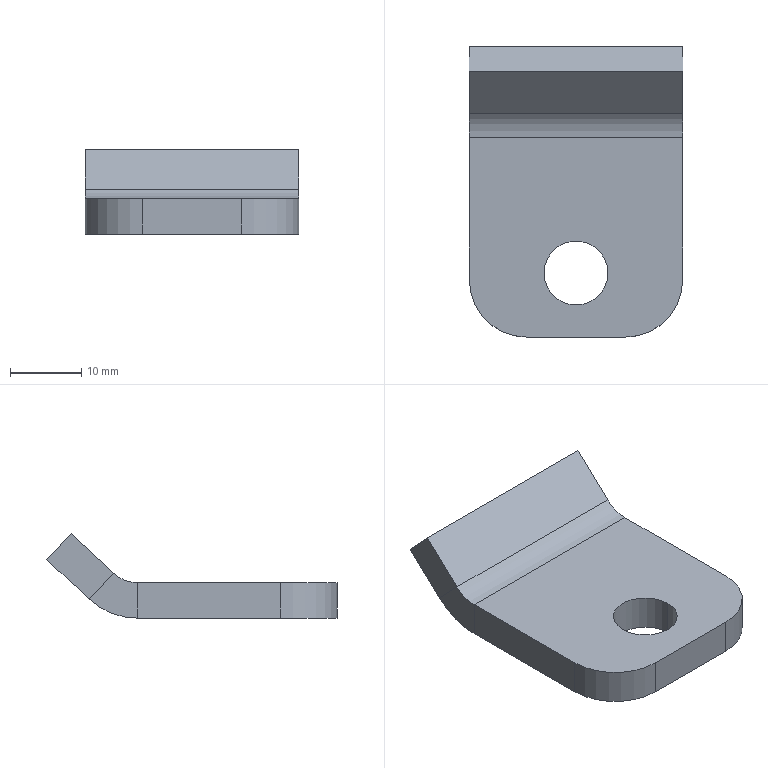Part | SolidWorks | features Fillet 1, FlatPattern 1, ICE 1, SMBaseFlange 1, SheetMetal 1 | 1 solid | 18 faces | box 30 x 40.8 x 11.858 mm | volume 5812 mm3 | plane 12 | cylinder 6 | commonest cylinder face diameters 9 x2 16 x2 10 x1 20 x1
STEP:
#1=CARTESIAN_POINT('',(19.5,9.,0.));
#2=VERTEX_POINT('',#1);
#3=CARTESIAN_POINT('',(10.5,9.,0.));
#4=VERTEX_POINT('',#3);
#5=CARTESIAN_POINT('',(15.,9.,0.));
#6=DIRECTION('',(0.,0.,-1.));
#7=DIRECTION('',(1.,0.,0.));
#8=AXIS2_PLACEMENT_3D('',#5,#6,#7);
#9=CIRCLE('',#8,4.5);
#10=EDGE_CURVE('',#2,#4,#9,.T.);
#11=ORIENTED_EDGE('',*,*,#10,.T.);
#12=CARTESIAN_POINT('',(10.5,9.,5.));
#13=VERTEX_POINT('',#12);
#14=CARTESIAN_POINT('',(10.5,9.,-0.001));
#15=DIRECTION('',(0.,0.,1.));
#16=VECTOR('',#15,1000.);
#17=LINE('',#14,#16);
#18=EDGE_CURVE('',#4,#13,#17,.T.);
#19=ORIENTED_EDGE('',*,*,#18,.T.);
#20=CARTESIAN_POINT('',(19.5,9.,5.));
#21=VERTEX_POINT('',#20);
#22=CARTESIAN_POINT('',(15.,9.,5.));
#23=DIRECTION('',(0.,0.,1.));
#24=DIRECTION('',(1.,0.,0.));
#25=AXIS2_PLACEMENT_3D('',#22,#23,#24);
#26=CIRCLE('',#25,4.5);
#27=EDGE_CURVE('',#13,#21,#26,.T.);
#28=ORIENTED_EDGE('',*,*,#27,.T.);
#29=CARTESIAN_POINT('',(19.5,9.,-0.001));
#30=DIRECTION('',(0.,0.,1.));
#31=VECTOR('',#30,1000.);
#32=LINE('',#29,#31);
#33=EDGE_CURVE('',#2,#21,#32,.T.);
#34=ORIENTED_EDGE('',*,*,#33,.F.);
#35=EDGE_LOOP('',(#11,#19,#28,#34));
#36=FACE_OUTER_BOUND('',#35,.T.);
#37=CARTESIAN_POINT('',(15.,9.,-0.001));
#38=DIRECTION('',(0.,0.,1.));
#39=DIRECTION('',(1.,0.,0.));
#40=AXIS2_PLACEMENT_3D('',#37,#38,#39);
#41=CYLINDRICAL_SURFACE('',#40,4.5);
#42=ADVANCED_FACE('',(#36),#41,.F.);
#43=CARTESIAN_POINT('',(30.,28.063,0.));
#44=VERTEX_POINT('',#43);
#45=CARTESIAN_POINT('',(30.,28.063,5.));
#46=VERTEX_POINT('',#45);
#47=CARTESIAN_POINT('',(30.,28.063,0.));
#48=DIRECTION('',(0.,0.,1.));
#49=VECTOR('',#48,1000.);
#50=LINE('',#47,#49);
#51=EDGE_CURVE('',#44,#46,#50,.T.);
#52=ORIENTED_EDGE('',*,*,#51,.F.);
#53=CARTESIAN_POINT('',(30.,34.88,2.684));
#54=VERTEX_POINT('',#53);
#55=CARTESIAN_POINT('',(30.,28.063,10.));
#56=DIRECTION('',(1.,0.,0.));
#57=DIRECTION('',(0.,0.,1.));
#58=AXIS2_PLACEMENT_3D('',#55,#56,#57);
#59=CIRCLE('',#58,10.);
#60=EDGE_CURVE('',#44,#54,#59,.T.);
#61=ORIENTED_EDGE('',*,*,#60,.T.);
#62=CARTESIAN_POINT('',(30.,31.472,6.342));
#63=VERTEX_POINT('',#62);
#64=CARTESIAN_POINT('',(30.,31.472,6.342));
#65=DIRECTION('',(0.,0.6817,-0.7316));
#66=VECTOR('',#65,1000.);
#67=LINE('',#64,#66);
#68=EDGE_CURVE('',#63,#54,#67,.T.);
#69=ORIENTED_EDGE('',*,*,#68,.F.);
#70=CARTESIAN_POINT('',(30.,28.063,10.));
#71=DIRECTION('',(1.,0.,0.));
#72=DIRECTION('',(0.,0.,-1.));
#73=AXIS2_PLACEMENT_3D('',#70,#71,#72);
#74=CIRCLE('',#73,5.);
#75=EDGE_CURVE('',#46,#63,#74,.T.);
#76=ORIENTED_EDGE('',*,*,#75,.F.);
#77=EDGE_LOOP('',(#52,#61,#69,#76));
#78=FACE_OUTER_BOUND('',#77,.T.);
#79=CARTESIAN_POINT('',(30.,28.063,0.));
#80=DIRECTION('',(1.,0.,0.));
#81=DIRECTION('',(0.,0.,-1.));
#82=AXIS2_PLACEMENT_3D('',#79,#80,#81);
#83=PLANE('',#82);
#84=ADVANCED_FACE('',(#78),#83,.T.);
#85=CARTESIAN_POINT('',(30.,8.,5.));
#86=VERTEX_POINT('',#85);
#87=CARTESIAN_POINT('',(30.,0.,5.));
#88=DIRECTION('',(0.,1.,0.));
#89=VECTOR('',#88,1000.);
#90=LINE('',#87,#89);
#91=EDGE_CURVE('',#86,#46,#90,.T.);
#92=ORIENTED_EDGE('',*,*,#91,.F.);
#93=CARTESIAN_POINT('',(30.,8.,0.));
#94=VERTEX_POINT('',#93);
#95=CARTESIAN_POINT('',(30.,8.,6.342));
#96=DIRECTION('',(0.,0.,-1.));
#97=VECTOR('',#96,1000.);
#98=LINE('',#95,#97);
#99=EDGE_CURVE('',#86,#94,#98,.T.);
#100=ORIENTED_EDGE('',*,*,#99,.T.);
#101=CARTESIAN_POINT('',(30.,0.,0.));
#102=DIRECTION('',(0.,1.,0.));
#103=VECTOR('',#102,1000.);
#104=LINE('',#101,#103);
#105=EDGE_CURVE('',#94,#44,#104,.T.);
#106=ORIENTED_EDGE('',*,*,#105,.T.);
#107=ORIENTED_EDGE('',*,*,#51,.T.);
#108=EDGE_LOOP('',(#92,#100,#106,#107));
#109=FACE_OUTER_BOUND('',#108,.T.);
#110=CARTESIAN_POINT('',(30.,31.472,6.342));
#111=DIRECTION('',(1.,0.,0.));
#112=DIRECTION('',(0.,0.,-1.));
#113=AXIS2_PLACEMENT_3D('',#110,#111,#112);
#114=PLANE('',#113);
#115=ADVANCED_FACE('',(#109),#114,.T.);
#116=CARTESIAN_POINT('',(0.,34.88,2.684));
#117=VERTEX_POINT('',#116);
#118=CARTESIAN_POINT('',(0.,31.472,6.342));
#119=VERTEX_POINT('',#118);
#120=CARTESIAN_POINT('',(0.,34.88,2.684));
#121=DIRECTION('',(0.,-0.6817,0.7316));
#122=VECTOR('',#121,1000.);
#123=LINE('',#120,#122);
#124=EDGE_CURVE('',#117,#119,#123,.T.);
#125=ORIENTED_EDGE('',*,*,#124,.F.);
#126=CARTESIAN_POINT('',(0.,28.063,0.));
#127=VERTEX_POINT('',#126);
#128=CARTESIAN_POINT('',(0.,28.063,10.));
#129=DIRECTION('',(1.,0.,0.));
#130=DIRECTION('',(0.,0.,1.));
#131=AXIS2_PLACEMENT_3D('',#128,#129,#130);
#132=CIRCLE('',#131,10.);
#133=EDGE_CURVE('',#127,#117,#132,.T.);
#134=ORIENTED_EDGE('',*,*,#133,.F.);
#135=CARTESIAN_POINT('',(0.,28.063,5.));
#136=VERTEX_POINT('',#135);
#137=CARTESIAN_POINT('',(0.,28.063,5.));
#138=DIRECTION('',(0.,0.,-1.));
#139=VECTOR('',#138,1000.);
#140=LINE('',#137,#139);
#141=EDGE_CURVE('',#136,#127,#140,.T.);
#142=ORIENTED_EDGE('',*,*,#141,.F.);
#143=CARTESIAN_POINT('',(0.,28.063,10.));
#144=DIRECTION('',(1.,0.,0.));
#145=DIRECTION('',(0.,0.,-1.));
#146=AXIS2_PLACEMENT_3D('',#143,#144,#145);
#147=CIRCLE('',#146,5.);
#148=EDGE_CURVE('',#136,#119,#147,.T.);
#149=ORIENTED_EDGE('',*,*,#148,.T.);
#150=EDGE_LOOP('',(#125,#134,#142,#149));
#151=FACE_OUTER_BOUND('',#150,.T.);
#152=CARTESIAN_POINT('',(0.,34.88,2.684));
#153=DIRECTION('',(-1.,0.,0.));
#154=DIRECTION('',(0.,0.,1.));
#155=AXIS2_PLACEMENT_3D('',#152,#153,#154);
#156=PLANE('',#155);
#157=ADVANCED_FACE('',(#151),#156,.T.);
#158=CARTESIAN_POINT('',(0.,40.8,8.2));
#159=VERTEX_POINT('',#158);
#160=CARTESIAN_POINT('',(0.,32.,0.));
#161=DIRECTION('',(0.,0.7316,0.6817));
#162=VECTOR('',#161,1000.);
#163=LINE('',#160,#162);
#164=EDGE_CURVE('',#117,#159,#163,.T.);
#165=ORIENTED_EDGE('',*,*,#164,.F.);
#166=ORIENTED_EDGE('',*,*,#124,.T.);
#167=CARTESIAN_POINT('',(0.,37.391,11.858));
#168=VERTEX_POINT('',#167);
#169=CARTESIAN_POINT('',(0.,28.591,3.658));
#170=DIRECTION('',(0.,0.7316,0.6817));
#171=VECTOR('',#170,1000.);
#172=LINE('',#169,#171);
#173=EDGE_CURVE('',#119,#168,#172,.T.);
#174=ORIENTED_EDGE('',*,*,#173,.T.);
#175=CARTESIAN_POINT('',(0.,37.391,11.858));
#176=DIRECTION('',(0.,0.6817,-0.7316));
#177=VECTOR('',#176,1000.);
#178=LINE('',#175,#177);
#179=EDGE_CURVE('',#168,#159,#178,.T.);
#180=ORIENTED_EDGE('',*,*,#179,.T.);
#181=EDGE_LOOP('',(#165,#166,#174,#180));
#182=FACE_OUTER_BOUND('',#181,.T.);
#183=CARTESIAN_POINT('',(0.,28.063,5.));
#184=DIRECTION('',(-1.,0.,0.));
#185=DIRECTION('',(0.,0.,1.));
#186=AXIS2_PLACEMENT_3D('',#183,#184,#185);
#187=PLANE('',#186);
#188=ADVANCED_FACE('',(#182),#187,.T.);
#189=ORIENTED_EDGE('',*,*,#164,.T.);
#190=CARTESIAN_POINT('',(30.,40.8,8.2));
#191=VERTEX_POINT('',#190);
#192=CARTESIAN_POINT('',(30.,40.8,8.2));
#193=DIRECTION('',(-1.,0.,0.));
#194=VECTOR('',#193,1000.);
#195=LINE('',#192,#194);
#196=EDGE_CURVE('',#191,#159,#195,.T.);
#197=ORIENTED_EDGE('',*,*,#196,.F.);
#198=CARTESIAN_POINT('',(30.,32.,0.));
#199=DIRECTION('',(0.,0.7316,0.6817));
#200=VECTOR('',#199,1000.);
#201=LINE('',#198,#200);
#202=EDGE_CURVE('',#54,#191,#201,.T.);
#203=ORIENTED_EDGE('',*,*,#202,.F.);
#204=CARTESIAN_POINT('',(30.,34.88,2.684));
#205=DIRECTION('',(-1.,0.,0.));
#206=VECTOR('',#205,1000.);
#207=LINE('',#204,#206);
#208=EDGE_CURVE('',#54,#117,#207,.T.);
#209=ORIENTED_EDGE('',*,*,#208,.T.);
#210=EDGE_LOOP('',(#189,#197,#203,#209));
#211=FACE_OUTER_BOUND('',#210,.T.);
#212=CARTESIAN_POINT('',(30.,32.,0.));
#213=DIRECTION('',(0.,-0.6817,0.7316));
#214=DIRECTION('',(0.,-0.7316,-0.6817));
#215=AXIS2_PLACEMENT_3D('',#212,#213,#214);
#216=PLANE('',#215);
#217=ADVANCED_FACE('',(#211),#216,.F.);
#218=ORIENTED_EDGE('',*,*,#179,.F.);
#219=CARTESIAN_POINT('',(30.,37.391,11.858));
#220=VERTEX_POINT('',#219);
#221=CARTESIAN_POINT('',(30.,37.391,11.858));
#222=DIRECTION('',(-1.,0.,0.));
#223=VECTOR('',#222,1000.);
#224=LINE('',#221,#223);
#225=EDGE_CURVE('',#220,#168,#224,.T.);
#226=ORIENTED_EDGE('',*,*,#225,.F.);
#227=CARTESIAN_POINT('',(30.,37.391,11.858));
#228=DIRECTION('',(0.,0.6817,-0.7316));
#229=VECTOR('',#228,1000.);
#230=LINE('',#227,#229);
#231=EDGE_CURVE('',#220,#191,#230,.T.);
#232=ORIENTED_EDGE('',*,*,#231,.T.);
#233=ORIENTED_EDGE('',*,*,#196,.T.);
#234=EDGE_LOOP('',(#218,#226,#232,#233));
#235=FACE_OUTER_BOUND('',#234,.T.);
#236=CARTESIAN_POINT('',(30.,37.391,11.858));
#237=DIRECTION('',(0.,0.7316,0.6817));
#238=DIRECTION('',(0.,-0.6817,0.7316));
#239=AXIS2_PLACEMENT_3D('',#236,#237,#238);
#240=PLANE('',#239);
#241=ADVANCED_FACE('',(#235),#240,.T.);
#242=ORIENTED_EDGE('',*,*,#173,.F.);
#243=CARTESIAN_POINT('',(30.,31.472,6.342));
#244=DIRECTION('',(-1.,0.,0.));
#245=VECTOR('',#244,1000.);
#246=LINE('',#243,#245);
#247=EDGE_CURVE('',#63,#119,#246,.T.);
#248=ORIENTED_EDGE('',*,*,#247,.F.);
#249=CARTESIAN_POINT('',(30.,28.591,3.658));
#250=DIRECTION('',(0.,0.7316,0.6817));
#251=VECTOR('',#250,1000.);
#252=LINE('',#249,#251);
#253=EDGE_CURVE('',#63,#220,#252,.T.);
#254=ORIENTED_EDGE('',*,*,#253,.T.);
#255=ORIENTED_EDGE('',*,*,#225,.T.);
#256=EDGE_LOOP('',(#242,#248,#254,#255));
#257=FACE_OUTER_BOUND('',#256,.T.);
#258=CARTESIAN_POINT('',(30.,28.591,3.658));
#259=DIRECTION('',(0.,-0.6817,0.7316));
#260=DIRECTION('',(0.,-0.7316,-0.6817));
#261=AXIS2_PLACEMENT_3D('',#258,#259,#260);
#262=PLANE('',#261);
#263=ADVANCED_FACE('',(#257),#262,.T.);
#264=ORIENTED_EDGE('',*,*,#148,.F.);
#265=CARTESIAN_POINT('',(30.,28.063,5.));
#266=DIRECTION('',(-1.,0.,0.));
#267=VECTOR('',#266,1000.);
#268=LINE('',#265,#267);
#269=EDGE_CURVE('',#46,#136,#268,.T.);
#270=ORIENTED_EDGE('',*,*,#269,.F.);
#271=ORIENTED_EDGE('',*,*,#75,.T.);
#272=ORIENTED_EDGE('',*,*,#247,.T.);
#273=EDGE_LOOP('',(#264,#270,#271,#272));
#274=FACE_OUTER_BOUND('',#273,.T.);
#275=CARTESIAN_POINT('',(30.,28.063,10.));
#276=DIRECTION('',(-1.,0.,0.));
#277=DIRECTION('',(0.,0.,1.));
#278=AXIS2_PLACEMENT_3D('',#275,#276,#277);
#279=CYLINDRICAL_SURFACE('',#278,5.);
#280=ADVANCED_FACE('',(#274),#279,.F.);
#281=CARTESIAN_POINT('',(15.,9.,5.));
#282=DIRECTION('',(0.,0.,1.));
#283=DIRECTION('',(1.,0.,0.));
#284=AXIS2_PLACEMENT_3D('',#281,#282,#283);
#285=CIRCLE('',#284,4.5);
#286=EDGE_CURVE('',#21,#13,#285,.T.);
#287=ORIENTED_EDGE('',*,*,#286,.F.);
#288=ORIENTED_EDGE('',*,*,#27,.F.);
#289=EDGE_LOOP('',(#287,#288));
#290=FACE_BOUND('',#289,.T.);
#291=CARTESIAN_POINT('',(0.,8.,5.));
#292=VERTEX_POINT('',#291);
#293=CARTESIAN_POINT('',(0.,0.,5.));
#294=DIRECTION('',(0.,1.,0.));
#295=VECTOR('',#294,1000.);
#296=LINE('',#293,#295);
#297=EDGE_CURVE('',#292,#136,#296,.T.);
#298=ORIENTED_EDGE('',*,*,#297,.F.);
#299=CARTESIAN_POINT('',(8.,0.,5.));
#300=VERTEX_POINT('',#299);
#301=CARTESIAN_POINT('',(8.,8.,5.));
#302=DIRECTION('',(0.,0.,1.));
#303=DIRECTION('',(1.,0.,0.));
#304=AXIS2_PLACEMENT_3D('',#301,#302,#303);
#305=CIRCLE('',#304,8.);
#306=EDGE_CURVE('',#292,#300,#305,.T.);
#307=ORIENTED_EDGE('',*,*,#306,.T.);
#308=CARTESIAN_POINT('',(22.,0.,5.));
#309=VERTEX_POINT('',#308);
#310=CARTESIAN_POINT('',(30.,0.,5.));
#311=DIRECTION('',(-1.,0.,0.));
#312=VECTOR('',#311,1000.);
#313=LINE('',#310,#312);
#314=EDGE_CURVE('',#309,#300,#313,.T.);
#315=ORIENTED_EDGE('',*,*,#314,.F.);
#316=CARTESIAN_POINT('',(22.,8.,5.));
#317=DIRECTION('',(0.,0.,1.));
#318=DIRECTION('',(1.,0.,0.));
#319=AXIS2_PLACEMENT_3D('',#316,#317,#318);
#320=CIRCLE('',#319,8.);
#321=EDGE_CURVE('',#309,#86,#320,.T.);
#322=ORIENTED_EDGE('',*,*,#321,.T.);
#323=ORIENTED_EDGE('',*,*,#91,.T.);
#324=ORIENTED_EDGE('',*,*,#269,.T.);
#325=EDGE_LOOP('',(#298,#307,#315,#322,#323,#324));
#326=FACE_OUTER_BOUND('',#325,.T.);
#327=CARTESIAN_POINT('',(30.,0.,5.));
#328=DIRECTION('',(0.,0.,1.));
#329=DIRECTION('',(1.,0.,0.));
#330=AXIS2_PLACEMENT_3D('',#327,#328,#329);
#331=PLANE('',#330);
#332=ADVANCED_FACE('',(#290,#326),#331,.T.);
#333=ORIENTED_EDGE('',*,*,#314,.T.);
#334=CARTESIAN_POINT('',(8.,0.,0.));
#335=VERTEX_POINT('',#334);
#336=CARTESIAN_POINT('',(8.,0.,0.));
#337=DIRECTION('',(0.,0.,-1.));
#338=VECTOR('',#337,1000.);
#339=LINE('',#336,#338);
#340=EDGE_CURVE('',#300,#335,#339,.T.);
#341=ORIENTED_EDGE('',*,*,#340,.T.);
#342=CARTESIAN_POINT('',(22.,0.,0.));
#343=VERTEX_POINT('',#342);
#344=CARTESIAN_POINT('',(30.,0.,0.));
#345=DIRECTION('',(-1.,0.,0.));
#346=VECTOR('',#345,1000.);
#347=LINE('',#344,#346);
#348=EDGE_CURVE('',#343,#335,#347,.T.);
#349=ORIENTED_EDGE('',*,*,#348,.F.);
#350=CARTESIAN_POINT('',(22.,0.,0.));
#351=DIRECTION('',(0.,0.,1.));
#352=VECTOR('',#351,1000.);
#353=LINE('',#350,#352);
#354=EDGE_CURVE('',#343,#309,#353,.T.);
#355=ORIENTED_EDGE('',*,*,#354,.T.);
#356=EDGE_LOOP('',(#333,#341,#349,#355));
#357=FACE_OUTER_BOUND('',#356,.T.);
#358=CARTESIAN_POINT('',(30.,0.,0.));
#359=DIRECTION('',(0.,-1.,0.));
#360=DIRECTION('',(0.,0.,-1.));
#361=AXIS2_PLACEMENT_3D('',#358,#359,#360);
#362=PLANE('',#361);
#363=ADVANCED_FACE('',(#357),#362,.T.);
#364=ORIENTED_EDGE('',*,*,#10,.F.);
#365=CARTESIAN_POINT('',(15.,9.,0.));
#366=DIRECTION('',(0.,0.,-1.));
#367=DIRECTION('',(1.,0.,0.));
#368=AXIS2_PLACEMENT_3D('',#365,#366,#367);
#369=CIRCLE('',#368,4.5);
#370=EDGE_CURVE('',#4,#2,#369,.T.);
#371=ORIENTED_EDGE('',*,*,#370,.F.);
#372=EDGE_LOOP('',(#364,#371));
#373=FACE_BOUND('',#372,.T.);
#374=ORIENTED_EDGE('',*,*,#348,.T.);
#375=CARTESIAN_POINT('',(0.,8.,0.));
#376=VERTEX_POINT('',#375);
#377=CARTESIAN_POINT('',(8.,8.,0.));
#378=DIRECTION('',(0.,0.,-1.));
#379=DIRECTION('',(1.,0.,0.));
#380=AXIS2_PLACEMENT_3D('',#377,#378,#379);
#381=CIRCLE('',#380,8.);
#382=EDGE_CURVE('',#335,#376,#381,.T.);
#383=ORIENTED_EDGE('',*,*,#382,.T.);
#384=CARTESIAN_POINT('',(0.,0.,0.));
#385=DIRECTION('',(0.,1.,0.));
#386=VECTOR('',#385,1000.);
#387=LINE('',#384,#386);
#388=EDGE_CURVE('',#376,#127,#387,.T.);
#389=ORIENTED_EDGE('',*,*,#388,.T.);
#390=CARTESIAN_POINT('',(30.,28.063,0.));
#391=DIRECTION('',(-1.,0.,0.));
#392=VECTOR('',#391,1000.);
#393=LINE('',#390,#392);
#394=EDGE_CURVE('',#44,#127,#393,.T.);
#395=ORIENTED_EDGE('',*,*,#394,.F.);
#396=ORIENTED_EDGE('',*,*,#105,.F.);
#397=CARTESIAN_POINT('',(22.,8.,0.));
#398=DIRECTION('',(0.,0.,-1.));
#399=DIRECTION('',(1.,0.,0.));
#400=AXIS2_PLACEMENT_3D('',#397,#398,#399);
#401=CIRCLE('',#400,8.);
#402=EDGE_CURVE('',#94,#343,#401,.T.);
#403=ORIENTED_EDGE('',*,*,#402,.T.);
#404=EDGE_LOOP('',(#374,#383,#389,#395,#396,#403));
#405=FACE_OUTER_BOUND('',#404,.T.);
#406=CARTESIAN_POINT('',(30.,0.,0.));
#407=DIRECTION('',(0.,0.,1.));
#408=DIRECTION('',(1.,0.,0.));
#409=AXIS2_PLACEMENT_3D('',#406,#407,#408);
#410=PLANE('',#409);
#411=ADVANCED_FACE('',(#373,#405),#410,.F.);
#412=ORIENTED_EDGE('',*,*,#133,.T.);
#413=ORIENTED_EDGE('',*,*,#208,.F.);
#414=ORIENTED_EDGE('',*,*,#60,.F.);
#415=ORIENTED_EDGE('',*,*,#394,.T.);
#416=EDGE_LOOP('',(#412,#413,#414,#415));
#417=FACE_OUTER_BOUND('',#416,.T.);
#418=CARTESIAN_POINT('',(30.,28.063,10.));
#419=DIRECTION('',(-1.,0.,0.));
#420=DIRECTION('',(0.,0.,1.));
#421=AXIS2_PLACEMENT_3D('',#418,#419,#420);
#422=CYLINDRICAL_SURFACE('',#421,10.);
#423=ADVANCED_FACE('',(#417),#422,.T.);
#424=ORIENTED_EDGE('',*,*,#202,.T.);
#425=ORIENTED_EDGE('',*,*,#231,.F.);
#426=ORIENTED_EDGE('',*,*,#253,.F.);
#427=ORIENTED_EDGE('',*,*,#68,.T.);
#428=EDGE_LOOP('',(#424,#425,#426,#427));
#429=FACE_OUTER_BOUND('',#428,.T.);
#430=CARTESIAN_POINT('',(30.,28.063,10.));
#431=DIRECTION('',(1.,0.,0.));
#432=DIRECTION('',(0.,0.,-1.));
#433=AXIS2_PLACEMENT_3D('',#430,#431,#432);
#434=PLANE('',#433);
#435=ADVANCED_FACE('',(#429),#434,.T.);
#436=ORIENTED_EDGE('',*,*,#388,.F.);
#437=CARTESIAN_POINT('',(0.,8.,5.));
#438=DIRECTION('',(0.,0.,1.));
#439=VECTOR('',#438,1000.);
#440=LINE('',#437,#439);
#441=EDGE_CURVE('',#376,#292,#440,.T.);
#442=ORIENTED_EDGE('',*,*,#441,.T.);
#443=ORIENTED_EDGE('',*,*,#297,.T.);
#444=ORIENTED_EDGE('',*,*,#141,.T.);
#445=EDGE_LOOP('',(#436,#442,#443,#444));
#446=FACE_OUTER_BOUND('',#445,.T.);
#447=CARTESIAN_POINT('',(0.,28.063,10.));
#448=DIRECTION('',(1.,0.,0.));
#449=DIRECTION('',(0.,0.,-1.));
#450=AXIS2_PLACEMENT_3D('',#447,#448,#449);
#451=PLANE('',#450);
#452=ADVANCED_FACE('',(#446),#451,.F.);
#453=ORIENTED_EDGE('',*,*,#18,.F.);
#454=ORIENTED_EDGE('',*,*,#370,.T.);
#455=ORIENTED_EDGE('',*,*,#33,.T.);
#456=ORIENTED_EDGE('',*,*,#286,.T.);
#457=EDGE_LOOP('',(#453,#454,#455,#456));
#458=FACE_OUTER_BOUND('',#457,.T.);
#459=CARTESIAN_POINT('',(15.,9.,-0.001));
#460=DIRECTION('',(0.,0.,1.));
#461=DIRECTION('',(1.,0.,0.));
#462=AXIS2_PLACEMENT_3D('',#459,#460,#461);
#463=CYLINDRICAL_SURFACE('',#462,4.5);
#464=ADVANCED_FACE('',(#458),#463,.F.);
#465=ORIENTED_EDGE('',*,*,#382,.F.);
#466=ORIENTED_EDGE('',*,*,#340,.F.);
#467=ORIENTED_EDGE('',*,*,#306,.F.);
#468=ORIENTED_EDGE('',*,*,#441,.F.);
#469=EDGE_LOOP('',(#465,#466,#467,#468));
#470=FACE_OUTER_BOUND('',#469,.T.);
#471=CARTESIAN_POINT('',(8.,8.,10.));
#472=DIRECTION('',(0.,0.,-1.));
#473=DIRECTION('',(-1.,0.,0.));
#474=AXIS2_PLACEMENT_3D('',#471,#472,#473);
#475=CYLINDRICAL_SURFACE('',#474,8.);
#476=ADVANCED_FACE('',(#470),#475,.T.);
#477=ORIENTED_EDGE('',*,*,#402,.F.);
#478=ORIENTED_EDGE('',*,*,#99,.F.);
#479=ORIENTED_EDGE('',*,*,#321,.F.);
#480=ORIENTED_EDGE('',*,*,#354,.F.);
#481=EDGE_LOOP('',(#477,#478,#479,#480));
#482=FACE_OUTER_BOUND('',#481,.T.);
#483=CARTESIAN_POINT('',(22.,8.,0.));
#484=DIRECTION('',(0.,0.,1.));
#485=DIRECTION('',(1.,0.,0.));
#486=AXIS2_PLACEMENT_3D('',#483,#484,#485);
#487=CYLINDRICAL_SURFACE('',#486,8.);
#488=ADVANCED_FACE('',(#482),#487,.T.);
#489=CLOSED_SHELL('',(#42,#84,#115,#157,#188,#217,#241,#263,#280,#332,#363,#411,#423,#435,#452,#464,#476,#488));
#490=MANIFOLD_SOLID_BREP('',#489);
#491=CARTESIAN_POINT('',(0.,0.,0.));
#492=DIRECTION('',(0.,0.,1.));
#493=DIRECTION('',(1.,0.,0.));
#494=AXIS2_PLACEMENT_3D('',#491,#492,#493);
#495=(LENGTH_UNIT()NAMED_UNIT(*)SI_UNIT(.MILLI.,.METRE.));
#496=UNCERTAINTY_MEASURE_WITH_UNIT(LENGTH_MEASURE(0.00001),#495,'','');
#497=(NAMED_UNIT(*)PLANE_ANGLE_UNIT()SI_UNIT($,.RADIAN.));
#498=(NAMED_UNIT(*)SI_UNIT($,.STERADIAN.)SOLID_ANGLE_UNIT());
#499=(GEOMETRIC_REPRESENTATION_CONTEXT(3)GLOBAL_UNCERTAINTY_ASSIGNED_CONTEXT((#496))GLOBAL_UNIT_ASSIGNED_CONTEXT((#495,#497,#498))REPRESENTATION_CONTEXT('',''));
#500=ADVANCED_BREP_SHAPE_REPRESENTATION('',(#490,#494),#499);